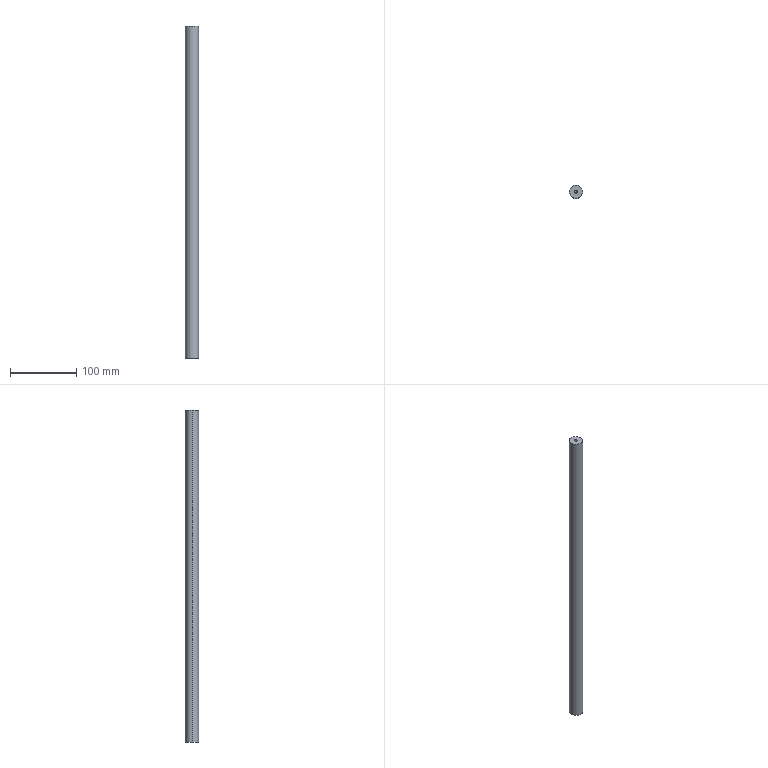Part | SolidWorks | features HoleWzd 2, Extrusion 1 | 1 solid | 12 faces | box 20 x 20 x 500 mm | volume 156724 mm3 | cylinder 6 | cone 4 | plane 2 | commonest cylinder face diameters 4.2 x4 20 x2
STEP:
#1=CARTESIAN_POINT('',(-2.1,0.,487.6));
#2=VERTEX_POINT('',#1);
#3=CARTESIAN_POINT('',(2.1,0.,487.6));
#4=VERTEX_POINT('',#3);
#5=CARTESIAN_POINT('',(0.,0.,487.6));
#6=DIRECTION('',(0.,0.,1.));
#7=DIRECTION('',(1.,0.,0.));
#8=AXIS2_PLACEMENT_3D('',#5,#6,#7);
#9=CIRCLE('',#8,2.1);
#10=EDGE_CURVE('',#2,#4,#9,.T.);
#11=ORIENTED_EDGE('',*,*,#10,.F.);
#12=CARTESIAN_POINT('',(-2.1,0.,500.));
#13=VERTEX_POINT('',#12);
#14=CARTESIAN_POINT('',(-2.1,0.,500.));
#15=DIRECTION('',(0.,0.,1.));
#16=VECTOR('',#15,1000.);
#17=LINE('',#14,#16);
#18=EDGE_CURVE('',#2,#13,#17,.T.);
#19=ORIENTED_EDGE('',*,*,#18,.T.);
#20=CARTESIAN_POINT('',(2.1,0.,500.));
#21=VERTEX_POINT('',#20);
#22=CARTESIAN_POINT('',(0.,0.,500.));
#23=DIRECTION('',(0.,0.,1.));
#24=DIRECTION('',(1.,0.,0.));
#25=AXIS2_PLACEMENT_3D('',#22,#23,#24);
#26=CIRCLE('',#25,2.1);
#27=EDGE_CURVE('',#13,#21,#26,.T.);
#28=ORIENTED_EDGE('',*,*,#27,.T.);
#29=CARTESIAN_POINT('',(2.1,0.,500.));
#30=DIRECTION('',(0.,0.,1.));
#31=VECTOR('',#30,1000.);
#32=LINE('',#29,#31);
#33=EDGE_CURVE('',#4,#21,#32,.T.);
#34=ORIENTED_EDGE('',*,*,#33,.F.);
#35=EDGE_LOOP('',(#11,#19,#28,#34));
#36=FACE_OUTER_BOUND('',#35,.T.);
#37=CARTESIAN_POINT('',(0.,0.,500.));
#38=DIRECTION('',(0.,0.,1.));
#39=DIRECTION('',(1.,0.,0.));
#40=AXIS2_PLACEMENT_3D('',#37,#38,#39);
#41=CYLINDRICAL_SURFACE('',#40,2.1);
#42=ADVANCED_FACE('',(#36),#41,.F.);
#43=CARTESIAN_POINT('',(0.,0.,486.338));
#44=VERTEX_POINT('',#43);
#45=CARTESIAN_POINT('',(2.1,0.,487.6));
#46=DIRECTION('',(0.8572,0.,0.515));
#47=VECTOR('',#46,1000.);
#48=LINE('',#45,#47);
#49=EDGE_CURVE('',#44,#4,#48,.T.);
#50=ORIENTED_EDGE('',*,*,#49,.F.);
#51=CARTESIAN_POINT('',(-2.1,0.,487.6));
#52=DIRECTION('',(-0.8572,0.,0.515));
#53=VECTOR('',#52,1000.);
#54=LINE('',#51,#53);
#55=EDGE_CURVE('',#44,#2,#54,.T.);
#56=ORIENTED_EDGE('',*,*,#55,.T.);
#57=ORIENTED_EDGE('',*,*,#10,.T.);
#58=EDGE_LOOP('',(#50,#56,#57));
#59=FACE_OUTER_BOUND('',#58,.T.);
#60=CARTESIAN_POINT('',(0.,0.,487.6));
#61=DIRECTION('',(0.,0.,1.));
#62=DIRECTION('',(1.,0.,0.));
#63=AXIS2_PLACEMENT_3D('',#60,#61,#62);
#64=CONICAL_SURFACE('',#63,2.1,1.03);
#65=ADVANCED_FACE('',(#59),#64,.F.);
#66=CARTESIAN_POINT('',(2.1,0.,12.4));
#67=VERTEX_POINT('',#66);
#68=CARTESIAN_POINT('',(-2.1,0.,12.4));
#69=VERTEX_POINT('',#68);
#70=CARTESIAN_POINT('',(0.,0.,12.4));
#71=DIRECTION('',(0.,0.,-1.));
#72=DIRECTION('',(-1.,0.,0.));
#73=AXIS2_PLACEMENT_3D('',#70,#71,#72);
#74=CIRCLE('',#73,2.1);
#75=EDGE_CURVE('',#67,#69,#74,.T.);
#76=ORIENTED_EDGE('',*,*,#75,.F.);
#77=CARTESIAN_POINT('',(2.1,0.,0.));
#78=VERTEX_POINT('',#77);
#79=CARTESIAN_POINT('',(2.1,0.,0.));
#80=DIRECTION('',(0.,0.,-1.));
#81=VECTOR('',#80,1000.);
#82=LINE('',#79,#81);
#83=EDGE_CURVE('',#67,#78,#82,.T.);
#84=ORIENTED_EDGE('',*,*,#83,.T.);
#85=CARTESIAN_POINT('',(-2.1,0.,0.));
#86=VERTEX_POINT('',#85);
#87=CARTESIAN_POINT('',(0.,0.,0.));
#88=DIRECTION('',(0.,0.,-1.));
#89=DIRECTION('',(-1.,0.,0.));
#90=AXIS2_PLACEMENT_3D('',#87,#88,#89);
#91=CIRCLE('',#90,2.1);
#92=EDGE_CURVE('',#78,#86,#91,.T.);
#93=ORIENTED_EDGE('',*,*,#92,.T.);
#94=CARTESIAN_POINT('',(-2.1,0.,0.));
#95=DIRECTION('',(0.,0.,-1.));
#96=VECTOR('',#95,1000.);
#97=LINE('',#94,#96);
#98=EDGE_CURVE('',#69,#86,#97,.T.);
#99=ORIENTED_EDGE('',*,*,#98,.F.);
#100=EDGE_LOOP('',(#76,#84,#93,#99));
#101=FACE_OUTER_BOUND('',#100,.T.);
#102=CARTESIAN_POINT('',(0.,0.,0.));
#103=DIRECTION('',(0.,0.,-1.));
#104=DIRECTION('',(-1.,0.,0.));
#105=AXIS2_PLACEMENT_3D('',#102,#103,#104);
#106=CYLINDRICAL_SURFACE('',#105,2.1);
#107=ADVANCED_FACE('',(#101),#106,.F.);
#108=CARTESIAN_POINT('',(0.,0.,13.662));
#109=VERTEX_POINT('',#108);
#110=CARTESIAN_POINT('',(-2.1,0.,12.4));
#111=DIRECTION('',(-0.8572,0.,-0.515));
#112=VECTOR('',#111,1000.);
#113=LINE('',#110,#112);
#114=EDGE_CURVE('',#109,#69,#113,.T.);
#115=ORIENTED_EDGE('',*,*,#114,.F.);
#116=CARTESIAN_POINT('',(2.1,0.,12.4));
#117=DIRECTION('',(0.8572,0.,-0.515));
#118=VECTOR('',#117,1000.);
#119=LINE('',#116,#118);
#120=EDGE_CURVE('',#109,#67,#119,.T.);
#121=ORIENTED_EDGE('',*,*,#120,.T.);
#122=ORIENTED_EDGE('',*,*,#75,.T.);
#123=EDGE_LOOP('',(#115,#121,#122));
#124=FACE_OUTER_BOUND('',#123,.T.);
#125=CARTESIAN_POINT('',(0.,0.,12.4));
#126=DIRECTION('',(0.,0.,-1.));
#127=DIRECTION('',(-1.,0.,0.));
#128=AXIS2_PLACEMENT_3D('',#125,#126,#127);
#129=CONICAL_SURFACE('',#128,2.1,1.03);
#130=ADVANCED_FACE('',(#124),#129,.F.);
#131=CARTESIAN_POINT('',(10.,0.,500.));
#132=VERTEX_POINT('',#131);
#133=CARTESIAN_POINT('',(-10.,0.,500.));
#134=VERTEX_POINT('',#133);
#135=CARTESIAN_POINT('',(0.,0.,500.));
#136=DIRECTION('',(0.,0.,1.));
#137=DIRECTION('',(1.,0.,0.));
#138=AXIS2_PLACEMENT_3D('',#135,#136,#137);
#139=CIRCLE('',#138,10.);
#140=EDGE_CURVE('',#132,#134,#139,.T.);
#141=ORIENTED_EDGE('',*,*,#140,.F.);
#142=CARTESIAN_POINT('',(10.,0.,0.));
#143=VERTEX_POINT('',#142);
#144=CARTESIAN_POINT('',(10.,0.,500.));
#145=DIRECTION('',(0.,0.,-1.));
#146=VECTOR('',#145,1000.);
#147=LINE('',#144,#146);
#148=EDGE_CURVE('',#132,#143,#147,.T.);
#149=ORIENTED_EDGE('',*,*,#148,.T.);
#150=CARTESIAN_POINT('',(-10.,0.,0.));
#151=VERTEX_POINT('',#150);
#152=CARTESIAN_POINT('',(0.,0.,0.));
#153=DIRECTION('',(0.,0.,1.));
#154=DIRECTION('',(1.,0.,0.));
#155=AXIS2_PLACEMENT_3D('',#152,#153,#154);
#156=CIRCLE('',#155,10.);
#157=EDGE_CURVE('',#143,#151,#156,.T.);
#158=ORIENTED_EDGE('',*,*,#157,.T.);
#159=CARTESIAN_POINT('',(-10.,0.,500.));
#160=DIRECTION('',(0.,0.,-1.));
#161=VECTOR('',#160,1000.);
#162=LINE('',#159,#161);
#163=EDGE_CURVE('',#134,#151,#162,.T.);
#164=ORIENTED_EDGE('',*,*,#163,.F.);
#165=EDGE_LOOP('',(#141,#149,#158,#164));
#166=FACE_OUTER_BOUND('',#165,.T.);
#167=CARTESIAN_POINT('',(0.,0.,500.));
#168=DIRECTION('',(0.,0.,-1.));
#169=DIRECTION('',(-1.,0.,0.));
#170=AXIS2_PLACEMENT_3D('',#167,#168,#169);
#171=CYLINDRICAL_SURFACE('',#170,10.);
#172=ADVANCED_FACE('',(#166),#171,.T.);
#173=ORIENTED_EDGE('',*,*,#148,.F.);
#174=CARTESIAN_POINT('',(0.,0.,500.));
#175=DIRECTION('',(0.,0.,1.));
#176=DIRECTION('',(1.,0.,0.));
#177=AXIS2_PLACEMENT_3D('',#174,#175,#176);
#178=CIRCLE('',#177,10.);
#179=EDGE_CURVE('',#134,#132,#178,.T.);
#180=ORIENTED_EDGE('',*,*,#179,.F.);
#181=ORIENTED_EDGE('',*,*,#163,.T.);
#182=CARTESIAN_POINT('',(0.,0.,0.));
#183=DIRECTION('',(0.,0.,1.));
#184=DIRECTION('',(1.,0.,0.));
#185=AXIS2_PLACEMENT_3D('',#182,#183,#184);
#186=CIRCLE('',#185,10.);
#187=EDGE_CURVE('',#151,#143,#186,.T.);
#188=ORIENTED_EDGE('',*,*,#187,.T.);
#189=EDGE_LOOP('',(#173,#180,#181,#188));
#190=FACE_OUTER_BOUND('',#189,.T.);
#191=CARTESIAN_POINT('',(0.,0.,500.));
#192=DIRECTION('',(0.,0.,-1.));
#193=DIRECTION('',(-1.,0.,0.));
#194=AXIS2_PLACEMENT_3D('',#191,#192,#193);
#195=CYLINDRICAL_SURFACE('',#194,10.);
#196=ADVANCED_FACE('',(#190),#195,.T.);
#197=CARTESIAN_POINT('',(0.,0.,500.));
#198=DIRECTION('',(0.,0.,1.));
#199=DIRECTION('',(1.,0.,0.));
#200=AXIS2_PLACEMENT_3D('',#197,#198,#199);
#201=CIRCLE('',#200,2.1);
#202=EDGE_CURVE('',#21,#13,#201,.T.);
#203=ORIENTED_EDGE('',*,*,#202,.F.);
#204=ORIENTED_EDGE('',*,*,#27,.F.);
#205=EDGE_LOOP('',(#203,#204));
#206=FACE_BOUND('',#205,.T.);
#207=ORIENTED_EDGE('',*,*,#179,.T.);
#208=ORIENTED_EDGE('',*,*,#140,.T.);
#209=EDGE_LOOP('',(#207,#208));
#210=FACE_OUTER_BOUND('',#209,.T.);
#211=CARTESIAN_POINT('',(0.,0.,500.));
#212=DIRECTION('',(0.,0.,1.));
#213=DIRECTION('',(1.,0.,0.));
#214=AXIS2_PLACEMENT_3D('',#211,#212,#213);
#215=PLANE('',#214);
#216=ADVANCED_FACE('',(#206,#210),#215,.T.);
#217=CARTESIAN_POINT('',(0.,0.,0.));
#218=DIRECTION('',(0.,0.,-1.));
#219=DIRECTION('',(-1.,0.,0.));
#220=AXIS2_PLACEMENT_3D('',#217,#218,#219);
#221=CIRCLE('',#220,2.1);
#222=EDGE_CURVE('',#86,#78,#221,.T.);
#223=ORIENTED_EDGE('',*,*,#222,.F.);
#224=ORIENTED_EDGE('',*,*,#92,.F.);
#225=EDGE_LOOP('',(#223,#224));
#226=FACE_BOUND('',#225,.T.);
#227=ORIENTED_EDGE('',*,*,#187,.F.);
#228=ORIENTED_EDGE('',*,*,#157,.F.);
#229=EDGE_LOOP('',(#227,#228));
#230=FACE_OUTER_BOUND('',#229,.T.);
#231=CARTESIAN_POINT('',(0.,0.,0.));
#232=DIRECTION('',(0.,0.,1.));
#233=DIRECTION('',(1.,0.,0.));
#234=AXIS2_PLACEMENT_3D('',#231,#232,#233);
#235=PLANE('',#234);
#236=ADVANCED_FACE('',(#226,#230),#235,.F.);
#237=ORIENTED_EDGE('',*,*,#120,.F.);
#238=ORIENTED_EDGE('',*,*,#114,.T.);
#239=CARTESIAN_POINT('',(0.,0.,12.4));
#240=DIRECTION('',(0.,0.,-1.));
#241=DIRECTION('',(-1.,0.,0.));
#242=AXIS2_PLACEMENT_3D('',#239,#240,#241);
#243=CIRCLE('',#242,2.1);
#244=EDGE_CURVE('',#69,#67,#243,.T.);
#245=ORIENTED_EDGE('',*,*,#244,.T.);
#246=EDGE_LOOP('',(#237,#238,#245));
#247=FACE_OUTER_BOUND('',#246,.T.);
#248=CARTESIAN_POINT('',(0.,0.,12.4));
#249=DIRECTION('',(0.,0.,-1.));
#250=DIRECTION('',(-1.,0.,0.));
#251=AXIS2_PLACEMENT_3D('',#248,#249,#250);
#252=CONICAL_SURFACE('',#251,2.1,1.03);
#253=ADVANCED_FACE('',(#247),#252,.F.);
#254=ORIENTED_EDGE('',*,*,#83,.F.);
#255=ORIENTED_EDGE('',*,*,#244,.F.);
#256=ORIENTED_EDGE('',*,*,#98,.T.);
#257=ORIENTED_EDGE('',*,*,#222,.T.);
#258=EDGE_LOOP('',(#254,#255,#256,#257));
#259=FACE_OUTER_BOUND('',#258,.T.);
#260=CARTESIAN_POINT('',(0.,0.,0.));
#261=DIRECTION('',(0.,0.,-1.));
#262=DIRECTION('',(-1.,0.,0.));
#263=AXIS2_PLACEMENT_3D('',#260,#261,#262);
#264=CYLINDRICAL_SURFACE('',#263,2.1);
#265=ADVANCED_FACE('',(#259),#264,.F.);
#266=ORIENTED_EDGE('',*,*,#55,.F.);
#267=ORIENTED_EDGE('',*,*,#49,.T.);
#268=CARTESIAN_POINT('',(0.,0.,487.6));
#269=DIRECTION('',(0.,0.,1.));
#270=DIRECTION('',(1.,0.,0.));
#271=AXIS2_PLACEMENT_3D('',#268,#269,#270);
#272=CIRCLE('',#271,2.1);
#273=EDGE_CURVE('',#4,#2,#272,.T.);
#274=ORIENTED_EDGE('',*,*,#273,.T.);
#275=EDGE_LOOP('',(#266,#267,#274));
#276=FACE_OUTER_BOUND('',#275,.T.);
#277=CARTESIAN_POINT('',(0.,0.,487.6));
#278=DIRECTION('',(0.,0.,1.));
#279=DIRECTION('',(1.,0.,0.));
#280=AXIS2_PLACEMENT_3D('',#277,#278,#279);
#281=CONICAL_SURFACE('',#280,2.1,1.03);
#282=ADVANCED_FACE('',(#276),#281,.F.);
#283=ORIENTED_EDGE('',*,*,#18,.F.);
#284=ORIENTED_EDGE('',*,*,#273,.F.);
#285=ORIENTED_EDGE('',*,*,#33,.T.);
#286=ORIENTED_EDGE('',*,*,#202,.T.);
#287=EDGE_LOOP('',(#283,#284,#285,#286));
#288=FACE_OUTER_BOUND('',#287,.T.);
#289=CARTESIAN_POINT('',(0.,0.,500.));
#290=DIRECTION('',(0.,0.,1.));
#291=DIRECTION('',(1.,0.,0.));
#292=AXIS2_PLACEMENT_3D('',#289,#290,#291);
#293=CYLINDRICAL_SURFACE('',#292,2.1);
#294=ADVANCED_FACE('',(#288),#293,.F.);
#295=CLOSED_SHELL('',(#42,#65,#107,#130,#172,#196,#216,#236,#253,#265,#282,#294));
#296=MANIFOLD_SOLID_BREP('',#295);
#297=CARTESIAN_POINT('',(0.,0.,0.));
#298=DIRECTION('',(0.,0.,1.));
#299=DIRECTION('',(1.,0.,0.));
#300=AXIS2_PLACEMENT_3D('',#297,#298,#299);
#301=(LENGTH_UNIT()NAMED_UNIT(*)SI_UNIT(.MILLI.,.METRE.));
#302=UNCERTAINTY_MEASURE_WITH_UNIT(LENGTH_MEASURE(0.00001),#301,'','');
#303=(NAMED_UNIT(*)PLANE_ANGLE_UNIT()SI_UNIT($,.RADIAN.));
#304=(NAMED_UNIT(*)SI_UNIT($,.STERADIAN.)SOLID_ANGLE_UNIT());
#305=(GEOMETRIC_REPRESENTATION_CONTEXT(3)GLOBAL_UNCERTAINTY_ASSIGNED_CONTEXT((#302))GLOBAL_UNIT_ASSIGNED_CONTEXT((#301,#303,#304))REPRESENTATION_CONTEXT('',''));
#306=ADVANCED_BREP_SHAPE_REPRESENTATION('',(#296,#300),#305);